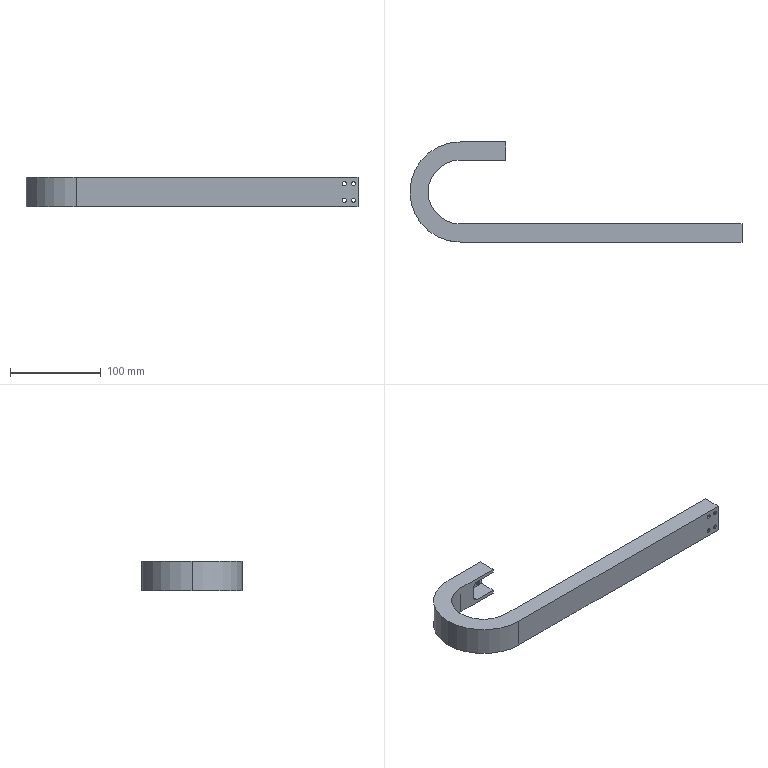Part | STEP file | Drag chain MHPKS203-45-15-A3 | 1 solid | 40 faces | box 365 x 110 x 32 mm | volume 295090 mm3 | cylinder 24 | plane 16 | commonest cylinder face diameters 4.5 x16 10 x4 70 x2 110 x2